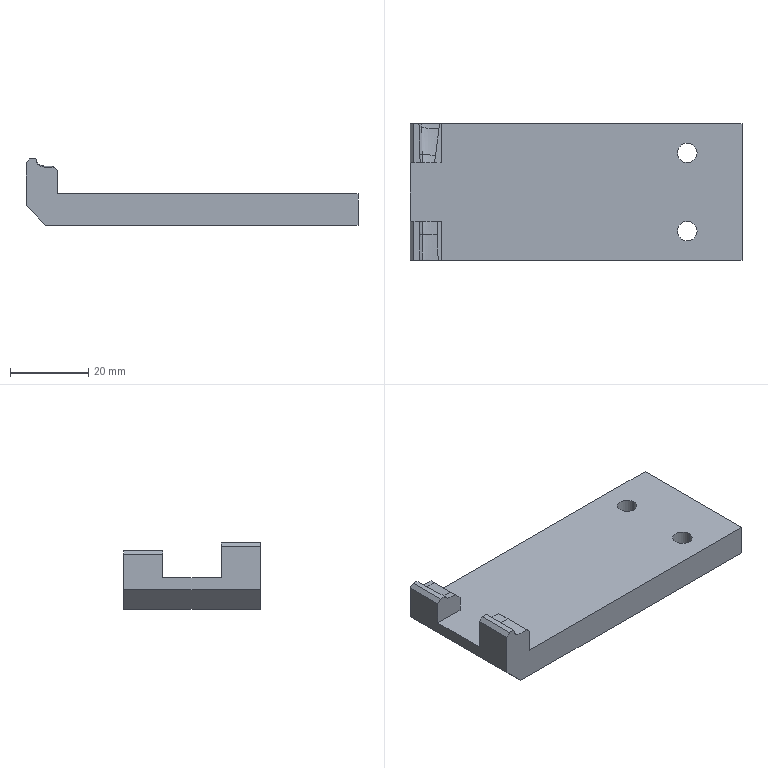Part | 1 solid | 31 faces | box 85 x 35 x 17 mm | volume 24108 mm3 | plane 17 | spline 10 | cylinder 4 | commonest cylinder face diameters 5 x4